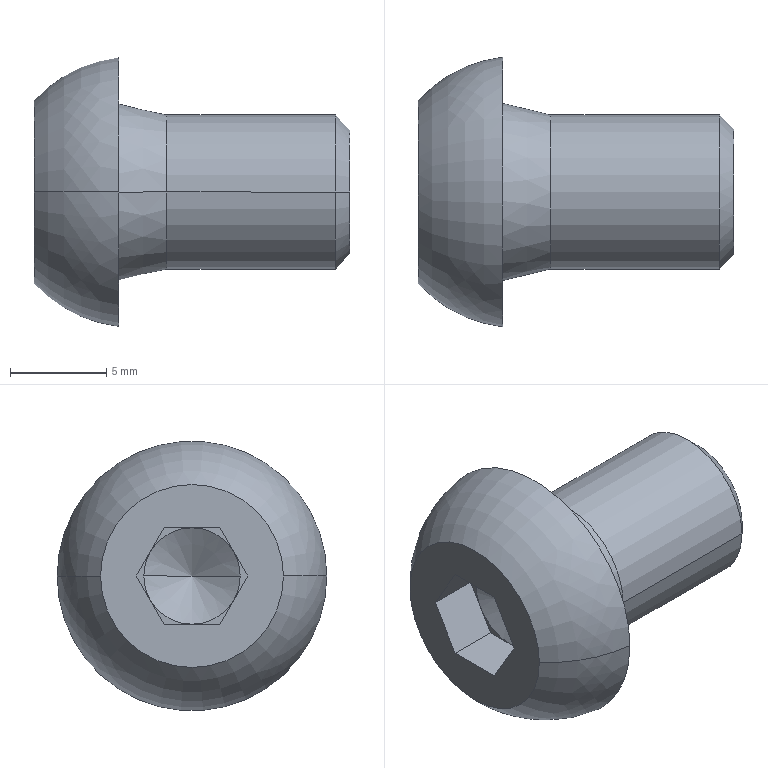Part | STEP file | M8x12 hex socket round-head bolt | 1 solid | 25 faces | box 16.4 x 14 x 14 mm | volume 1090 mm3 | plane 15 | cone 6 | other 2 | cylinder 2 | commonest cylinder face diameters 8 x2